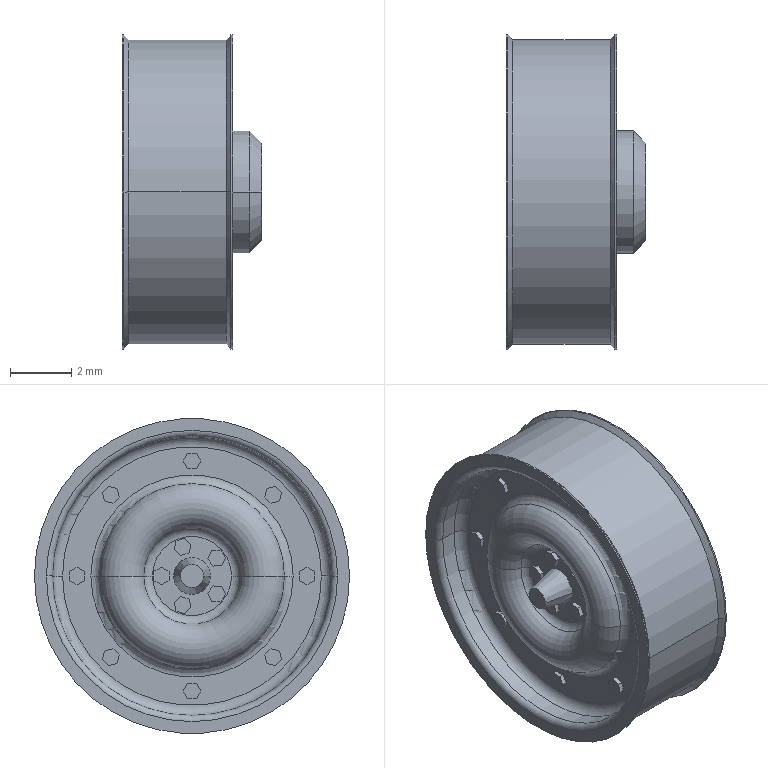Part | SolidWorks | features Chamfer 2, CirPattern 2, ICE 2, Fillet 1, Revolution 1 | 1 solid | 133 faces | box 4.55 x 10.3 x 10.3 mm | volume 146.742 mm3 | plane 99 | cylinder 14 | cone 10 | torus 10 | commonest cylinder face diameters 9.121 x4 10.3 x4 1.5 x2 4 x2 9.966 x2